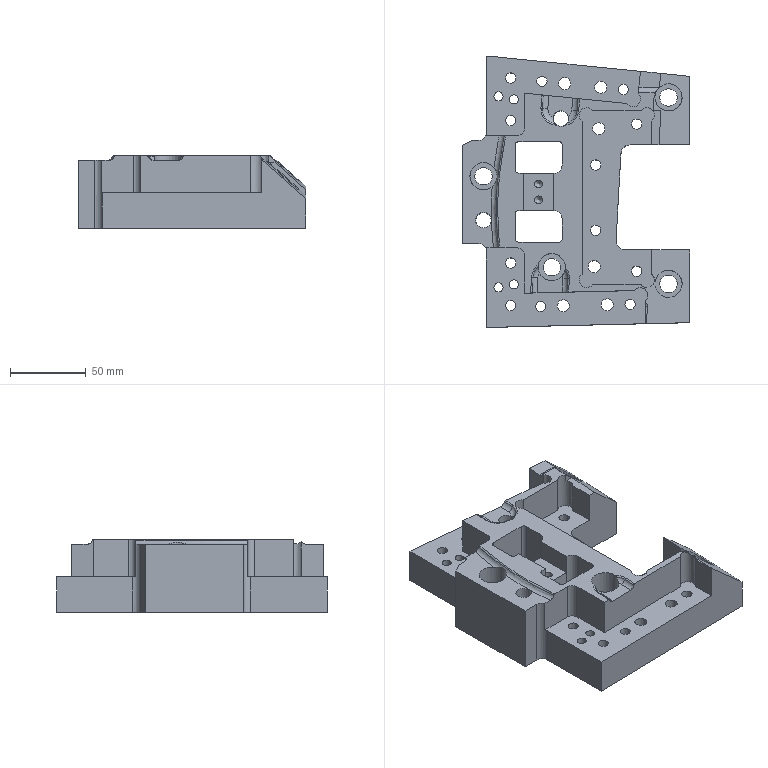Part | NX | features solid 2 | 1 solid | 133 faces | box 150 x 178.728 x 48 mm | volume 579726 mm3 | cylinder 65 | plane 55 | torus 10 | cone 2 | spline 1 | commonest cylinder face diameters 6.8 x12 10 x8 5 x6 8.001 x6 2 x4 6.001 x4